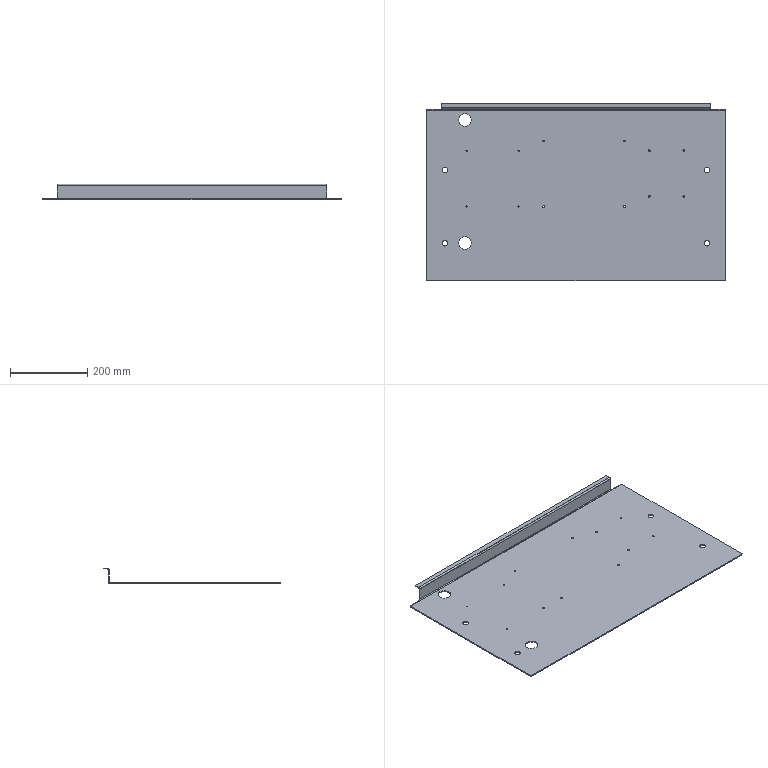Part | NX | features solid 2 | 1 solid | 68 faces | box 776 x 461.5 x 40.5 mm | volume 1100110 mm3 | cylinder 44 | plane 24 | commonest cylinder face diameters 4.917 x16 3.2 x8 15 x8 6 x4 33 x4 4 x2